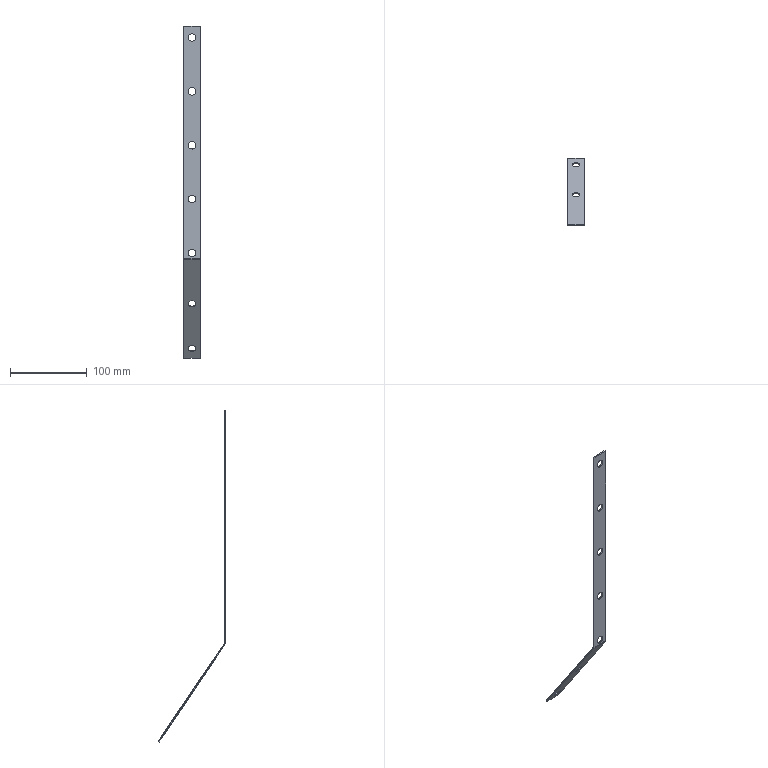Part | SolidWorks | features ICE 2, FlatPattern 1, SMBaseFlange 1, SheetMetal 1 | 1 solid | 28 faces | box 22 x 88.001 x 431.5 mm | volume 15223 mm3 | cylinder 16 | plane 12 | commonest cylinder face diameters 10 x14 3 x1 6.2 x1
STEP:
#1=CARTESIAN_POINT('',(0.,81.083,-120.21));
#2=VERTEX_POINT('',#1);
#3=CARTESIAN_POINT('',(0.,75.491,-111.92));
#4=VERTEX_POINT('',#3);
#5=CARTESIAN_POINT('',(0.,78.287,-116.065));
#6=DIRECTION('',(0.,0.829,0.5592));
#7=DIRECTION('',(0.,-0.5592,0.829));
#8=AXIS2_PLACEMENT_3D('',#5,#6,#7);
#9=CIRCLE('',#8,5.);
#10=EDGE_CURVE('',#2,#4,#9,.T.);
#11=ORIENTED_EDGE('',*,*,#10,.F.);
#12=CARTESIAN_POINT('',(0.,82.409,-119.316));
#13=VERTEX_POINT('',#12);
#14=CARTESIAN_POINT('',(0.,21.511,-160.392));
#15=DIRECTION('',(0.,0.829,0.5592));
#16=VECTOR('',#15,1000.);
#17=LINE('',#14,#16);
#18=EDGE_CURVE('',#2,#13,#17,.T.);
#19=ORIENTED_EDGE('',*,*,#18,.T.);
#20=CARTESIAN_POINT('',(0.,76.818,-111.025));
#21=VERTEX_POINT('',#20);
#22=CARTESIAN_POINT('',(0.,79.613,-115.171));
#23=DIRECTION('',(0.,0.829,0.5592));
#24=DIRECTION('',(0.,-0.5592,0.829));
#25=AXIS2_PLACEMENT_3D('',#22,#23,#24);
#26=CIRCLE('',#25,5.);
#27=EDGE_CURVE('',#13,#21,#26,.T.);
#28=ORIENTED_EDGE('',*,*,#27,.T.);
#29=CARTESIAN_POINT('',(0.,15.919,-152.102));
#30=DIRECTION('',(0.,0.829,0.5592));
#31=VECTOR('',#30,1000.);
#32=LINE('',#29,#31);
#33=EDGE_CURVE('',#4,#21,#32,.T.);
#34=ORIENTED_EDGE('',*,*,#33,.F.);
#35=EDGE_LOOP('',(#11,#19,#28,#34));
#36=FACE_OUTER_BOUND('',#35,.T.);
#37=CARTESIAN_POINT('',(0.,18.715,-156.247));
#38=DIRECTION('',(0.,0.829,0.5592));
#39=DIRECTION('',(0.,-0.5592,0.829));
#40=AXIS2_PLACEMENT_3D('',#37,#38,#39);
#41=CYLINDRICAL_SURFACE('',#40,5.);
#42=ADVANCED_FACE('',(#36),#41,.F.);
#43=CARTESIAN_POINT('',(0.,41.939,-62.178));
#44=VERTEX_POINT('',#43);
#45=CARTESIAN_POINT('',(0.,36.348,-53.887));
#46=VERTEX_POINT('',#45);
#47=CARTESIAN_POINT('',(0.,39.144,-58.033));
#48=DIRECTION('',(0.,0.829,0.5592));
#49=DIRECTION('',(0.,-0.5592,0.829));
#50=AXIS2_PLACEMENT_3D('',#47,#48,#49);
#51=CIRCLE('',#50,5.);
#52=EDGE_CURVE('',#44,#46,#51,.T.);
#53=ORIENTED_EDGE('',*,*,#52,.F.);
#54=CARTESIAN_POINT('',(0.,43.266,-61.283));
#55=VERTEX_POINT('',#54);
#56=CARTESIAN_POINT('',(0.,-17.632,-102.359));
#57=DIRECTION('',(0.,0.829,0.5592));
#58=VECTOR('',#57,1000.);
#59=LINE('',#56,#58);
#60=EDGE_CURVE('',#44,#55,#59,.T.);
#61=ORIENTED_EDGE('',*,*,#60,.T.);
#62=CARTESIAN_POINT('',(0.,37.674,-52.993));
#63=VERTEX_POINT('',#62);
#64=CARTESIAN_POINT('',(0.,40.47,-57.138));
#65=DIRECTION('',(0.,0.829,0.5592));
#66=DIRECTION('',(0.,-0.5592,0.829));
#67=AXIS2_PLACEMENT_3D('',#64,#65,#66);
#68=CIRCLE('',#67,5.);
#69=EDGE_CURVE('',#55,#63,#68,.T.);
#70=ORIENTED_EDGE('',*,*,#69,.T.);
#71=CARTESIAN_POINT('',(0.,-23.224,-94.069));
#72=DIRECTION('',(0.,0.829,0.5592));
#73=VECTOR('',#72,1000.);
#74=LINE('',#71,#73);
#75=EDGE_CURVE('',#46,#63,#74,.T.);
#76=ORIENTED_EDGE('',*,*,#75,.F.);
#77=EDGE_LOOP('',(#53,#61,#70,#76));
#78=FACE_OUTER_BOUND('',#77,.T.);
#79=CARTESIAN_POINT('',(0.,-20.428,-98.214));
#80=DIRECTION('',(0.,0.829,0.5592));
#81=DIRECTION('',(0.,-0.5592,0.829));
#82=AXIS2_PLACEMENT_3D('',#79,#80,#81);
#83=CYLINDRICAL_SURFACE('',#82,5.);
#84=ADVANCED_FACE('',(#78),#83,.F.);
#85=CARTESIAN_POINT('',(0.,0.,283.));
#86=VERTEX_POINT('',#85);
#87=CARTESIAN_POINT('',(0.,0.,293.));
#88=VERTEX_POINT('',#87);
#89=CARTESIAN_POINT('',(0.,0.,288.));
#90=DIRECTION('',(0.,1.,0.));
#91=DIRECTION('',(0.,0.,1.));
#92=AXIS2_PLACEMENT_3D('',#89,#90,#91);
#93=CIRCLE('',#92,5.);
#94=EDGE_CURVE('',#86,#88,#93,.T.);
#95=ORIENTED_EDGE('',*,*,#94,.F.);
#96=CARTESIAN_POINT('',(0.,1.6,283.));
#97=VERTEX_POINT('',#96);
#98=CARTESIAN_POINT('',(0.,0.,283.));
#99=DIRECTION('',(0.,1.,0.));
#100=VECTOR('',#99,1000.);
#101=LINE('',#98,#100);
#102=EDGE_CURVE('',#86,#97,#101,.T.);
#103=ORIENTED_EDGE('',*,*,#102,.T.);
#104=CARTESIAN_POINT('',(0.,1.6,293.));
#105=VERTEX_POINT('',#104);
#106=CARTESIAN_POINT('',(0.,1.6,288.));
#107=DIRECTION('',(0.,1.,0.));
#108=DIRECTION('',(0.,0.,1.));
#109=AXIS2_PLACEMENT_3D('',#106,#107,#108);
#110=CIRCLE('',#109,5.);
#111=EDGE_CURVE('',#97,#105,#110,.T.);
#112=ORIENTED_EDGE('',*,*,#111,.T.);
#113=CARTESIAN_POINT('',(0.,0.,293.));
#114=DIRECTION('',(0.,1.,0.));
#115=VECTOR('',#114,1000.);
#116=LINE('',#113,#115);
#117=EDGE_CURVE('',#88,#105,#116,.T.);
#118=ORIENTED_EDGE('',*,*,#117,.F.);
#119=EDGE_LOOP('',(#95,#103,#112,#118));
#120=FACE_OUTER_BOUND('',#119,.T.);
#121=CARTESIAN_POINT('',(0.,0.,288.));
#122=DIRECTION('',(0.,1.,0.));
#123=DIRECTION('',(0.,0.,1.));
#124=AXIS2_PLACEMENT_3D('',#121,#122,#123);
#125=CYLINDRICAL_SURFACE('',#124,5.);
#126=ADVANCED_FACE('',(#120),#125,.F.);
#127=CARTESIAN_POINT('',(0.,0.,213.));
#128=VERTEX_POINT('',#127);
#129=CARTESIAN_POINT('',(0.,0.,223.));
#130=VERTEX_POINT('',#129);
#131=CARTESIAN_POINT('',(0.,0.,218.));
#132=DIRECTION('',(0.,1.,0.));
#133=DIRECTION('',(0.,0.,1.));
#134=AXIS2_PLACEMENT_3D('',#131,#132,#133);
#135=CIRCLE('',#134,5.);
#136=EDGE_CURVE('',#128,#130,#135,.T.);
#137=ORIENTED_EDGE('',*,*,#136,.F.);
#138=CARTESIAN_POINT('',(0.,1.6,213.));
#139=VERTEX_POINT('',#138);
#140=CARTESIAN_POINT('',(0.,0.,213.));
#141=DIRECTION('',(0.,1.,0.));
#142=VECTOR('',#141,1000.);
#143=LINE('',#140,#142);
#144=EDGE_CURVE('',#128,#139,#143,.T.);
#145=ORIENTED_EDGE('',*,*,#144,.T.);
#146=CARTESIAN_POINT('',(0.,1.6,223.));
#147=VERTEX_POINT('',#146);
#148=CARTESIAN_POINT('',(0.,1.6,218.));
#149=DIRECTION('',(0.,1.,0.));
#150=DIRECTION('',(0.,0.,1.));
#151=AXIS2_PLACEMENT_3D('',#148,#149,#150);
#152=CIRCLE('',#151,5.);
#153=EDGE_CURVE('',#139,#147,#152,.T.);
#154=ORIENTED_EDGE('',*,*,#153,.T.);
#155=CARTESIAN_POINT('',(0.,0.,223.));
#156=DIRECTION('',(0.,1.,0.));
#157=VECTOR('',#156,1000.);
#158=LINE('',#155,#157);
#159=EDGE_CURVE('',#130,#147,#158,.T.);
#160=ORIENTED_EDGE('',*,*,#159,.F.);
#161=EDGE_LOOP('',(#137,#145,#154,#160));
#162=FACE_OUTER_BOUND('',#161,.T.);
#163=CARTESIAN_POINT('',(0.,0.,218.));
#164=DIRECTION('',(0.,1.,0.));
#165=DIRECTION('',(0.,0.,1.));
#166=AXIS2_PLACEMENT_3D('',#163,#164,#165);
#167=CYLINDRICAL_SURFACE('',#166,5.);
#168=ADVANCED_FACE('',(#162),#167,.F.);
#169=CARTESIAN_POINT('',(0.,0.,143.));
#170=VERTEX_POINT('',#169);
#171=CARTESIAN_POINT('',(0.,0.,153.));
#172=VERTEX_POINT('',#171);
#173=CARTESIAN_POINT('',(0.,0.,148.));
#174=DIRECTION('',(0.,1.,0.));
#175=DIRECTION('',(0.,0.,1.));
#176=AXIS2_PLACEMENT_3D('',#173,#174,#175);
#177=CIRCLE('',#176,5.);
#178=EDGE_CURVE('',#170,#172,#177,.T.);
#179=ORIENTED_EDGE('',*,*,#178,.F.);
#180=CARTESIAN_POINT('',(0.,1.6,143.));
#181=VERTEX_POINT('',#180);
#182=CARTESIAN_POINT('',(0.,0.,143.));
#183=DIRECTION('',(0.,1.,0.));
#184=VECTOR('',#183,1000.);
#185=LINE('',#182,#184);
#186=EDGE_CURVE('',#170,#181,#185,.T.);
#187=ORIENTED_EDGE('',*,*,#186,.T.);
#188=CARTESIAN_POINT('',(0.,1.6,153.));
#189=VERTEX_POINT('',#188);
#190=CARTESIAN_POINT('',(0.,1.6,148.));
#191=DIRECTION('',(0.,1.,0.));
#192=DIRECTION('',(0.,0.,1.));
#193=AXIS2_PLACEMENT_3D('',#190,#191,#192);
#194=CIRCLE('',#193,5.);
#195=EDGE_CURVE('',#181,#189,#194,.T.);
#196=ORIENTED_EDGE('',*,*,#195,.T.);
#197=CARTESIAN_POINT('',(0.,0.,153.));
#198=DIRECTION('',(0.,1.,0.));
#199=VECTOR('',#198,1000.);
#200=LINE('',#197,#199);
#201=EDGE_CURVE('',#172,#189,#200,.T.);
#202=ORIENTED_EDGE('',*,*,#201,.F.);
#203=EDGE_LOOP('',(#179,#187,#196,#202));
#204=FACE_OUTER_BOUND('',#203,.T.);
#205=CARTESIAN_POINT('',(0.,0.,148.));
#206=DIRECTION('',(0.,1.,0.));
#207=DIRECTION('',(0.,0.,1.));
#208=AXIS2_PLACEMENT_3D('',#205,#206,#207);
#209=CYLINDRICAL_SURFACE('',#208,5.);
#210=ADVANCED_FACE('',(#204),#209,.F.);
#211=CARTESIAN_POINT('',(0.,0.,73.));
#212=VERTEX_POINT('',#211);
#213=CARTESIAN_POINT('',(0.,0.,83.));
#214=VERTEX_POINT('',#213);
#215=CARTESIAN_POINT('',(0.,0.,78.));
#216=DIRECTION('',(0.,1.,0.));
#217=DIRECTION('',(0.,0.,1.));
#218=AXIS2_PLACEMENT_3D('',#215,#216,#217);
#219=CIRCLE('',#218,5.);
#220=EDGE_CURVE('',#212,#214,#219,.T.);
#221=ORIENTED_EDGE('',*,*,#220,.F.);
#222=CARTESIAN_POINT('',(0.,1.6,73.));
#223=VERTEX_POINT('',#222);
#224=CARTESIAN_POINT('',(0.,0.,73.));
#225=DIRECTION('',(0.,1.,0.));
#226=VECTOR('',#225,1000.);
#227=LINE('',#224,#226);
#228=EDGE_CURVE('',#212,#223,#227,.T.);
#229=ORIENTED_EDGE('',*,*,#228,.T.);
#230=CARTESIAN_POINT('',(0.,1.6,83.));
#231=VERTEX_POINT('',#230);
#232=CARTESIAN_POINT('',(0.,1.6,78.));
#233=DIRECTION('',(0.,1.,0.));
#234=DIRECTION('',(0.,0.,1.));
#235=AXIS2_PLACEMENT_3D('',#232,#233,#234);
#236=CIRCLE('',#235,5.);
#237=EDGE_CURVE('',#223,#231,#236,.T.);
#238=ORIENTED_EDGE('',*,*,#237,.T.);
#239=CARTESIAN_POINT('',(0.,0.,83.));
#240=DIRECTION('',(0.,1.,0.));
#241=VECTOR('',#240,1000.);
#242=LINE('',#239,#241);
#243=EDGE_CURVE('',#214,#231,#242,.T.);
#244=ORIENTED_EDGE('',*,*,#243,.F.);
#245=EDGE_LOOP('',(#221,#229,#238,#244));
#246=FACE_OUTER_BOUND('',#245,.T.);
#247=CARTESIAN_POINT('',(0.,0.,78.));
#248=DIRECTION('',(0.,1.,0.));
#249=DIRECTION('',(0.,0.,1.));
#250=AXIS2_PLACEMENT_3D('',#247,#248,#249);
#251=CYLINDRICAL_SURFACE('',#250,5.);
#252=ADVANCED_FACE('',(#246),#251,.F.);
#253=CARTESIAN_POINT('',(0.,0.,3.));
#254=VERTEX_POINT('',#253);
#255=CARTESIAN_POINT('',(0.,0.,13.));
#256=VERTEX_POINT('',#255);
#257=CARTESIAN_POINT('',(0.,0.,8.));
#258=DIRECTION('',(0.,1.,0.));
#259=DIRECTION('',(0.,0.,1.));
#260=AXIS2_PLACEMENT_3D('',#257,#258,#259);
#261=CIRCLE('',#260,5.);
#262=EDGE_CURVE('',#254,#256,#261,.T.);
#263=ORIENTED_EDGE('',*,*,#262,.F.);
#264=CARTESIAN_POINT('',(0.,1.6,3.));
#265=VERTEX_POINT('',#264);
#266=CARTESIAN_POINT('',(0.,0.,3.));
#267=DIRECTION('',(0.,1.,0.));
#268=VECTOR('',#267,1000.);
#269=LINE('',#266,#268);
#270=EDGE_CURVE('',#254,#265,#269,.T.);
#271=ORIENTED_EDGE('',*,*,#270,.T.);
#272=CARTESIAN_POINT('',(0.,1.6,13.));
#273=VERTEX_POINT('',#272);
#274=CARTESIAN_POINT('',(0.,1.6,8.));
#275=DIRECTION('',(0.,1.,0.));
#276=DIRECTION('',(0.,0.,1.));
#277=AXIS2_PLACEMENT_3D('',#274,#275,#276);
#278=CIRCLE('',#277,5.);
#279=EDGE_CURVE('',#265,#273,#278,.T.);
#280=ORIENTED_EDGE('',*,*,#279,.T.);
#281=CARTESIAN_POINT('',(0.,0.,13.));
#282=DIRECTION('',(0.,1.,0.));
#283=VECTOR('',#282,1000.);
#284=LINE('',#281,#283);
#285=EDGE_CURVE('',#256,#273,#284,.T.);
#286=ORIENTED_EDGE('',*,*,#285,.F.);
#287=EDGE_LOOP('',(#263,#271,#280,#286));
#288=FACE_OUTER_BOUND('',#287,.T.);
#289=CARTESIAN_POINT('',(0.,0.,8.));
#290=DIRECTION('',(0.,1.,0.));
#291=DIRECTION('',(0.,0.,1.));
#292=AXIS2_PLACEMENT_3D('',#289,#290,#291);
#293=CYLINDRICAL_SURFACE('',#292,5.);
#294=ADVANCED_FACE('',(#288),#293,.F.);
#295=CARTESIAN_POINT('',(11.,0.,0.9478));
#296=VERTEX_POINT('',#295);
#297=CARTESIAN_POINT('',(11.,1.6,0.9478));
#298=VERTEX_POINT('',#297);
#299=CARTESIAN_POINT('',(11.,0.,0.9478));
#300=DIRECTION('',(0.,1.,0.));
#301=VECTOR('',#300,1000.);
#302=LINE('',#299,#301);
#303=EDGE_CURVE('',#296,#298,#302,.T.);
#304=ORIENTED_EDGE('',*,*,#303,.F.);
#305=CARTESIAN_POINT('',(11.,0.53,-0.7857));
#306=VERTEX_POINT('',#305);
#307=CARTESIAN_POINT('',(11.,3.1,0.9478));
#308=DIRECTION('',(1.,0.,0.));
#309=DIRECTION('',(0.,0.,1.));
#310=AXIS2_PLACEMENT_3D('',#307,#308,#309);
#311=CIRCLE('',#310,3.1);
#312=EDGE_CURVE('',#296,#306,#311,.T.);
#313=ORIENTED_EDGE('',*,*,#312,.T.);
#314=CARTESIAN_POINT('',(11.,1.856,0.109));
#315=VERTEX_POINT('',#314);
#316=CARTESIAN_POINT('',(11.,1.856,0.109));
#317=DIRECTION('',(0.,-0.829,-0.5592));
#318=VECTOR('',#317,1000.);
#319=LINE('',#316,#318);
#320=EDGE_CURVE('',#315,#306,#319,.T.);
#321=ORIENTED_EDGE('',*,*,#320,.F.);
#322=CARTESIAN_POINT('',(11.,3.1,0.9478));
#323=DIRECTION('',(1.,0.,0.));
#324=DIRECTION('',(0.,0.,-1.));
#325=AXIS2_PLACEMENT_3D('',#322,#323,#324);
#326=CIRCLE('',#325,1.5);
#327=EDGE_CURVE('',#298,#315,#326,.T.);
#328=ORIENTED_EDGE('',*,*,#327,.F.);
#329=EDGE_LOOP('',(#304,#313,#321,#328));
#330=FACE_OUTER_BOUND('',#329,.T.);
#331=CARTESIAN_POINT('',(11.,0.,0.9478));
#332=DIRECTION('',(1.,0.,0.));
#333=DIRECTION('',(0.,0.,-1.));
#334=AXIS2_PLACEMENT_3D('',#331,#332,#333);
#335=PLANE('',#334);
#336=ADVANCED_FACE('',(#330),#335,.T.);
#337=CARTESIAN_POINT('',(11.,0.,303.));
#338=VERTEX_POINT('',#337);
#339=CARTESIAN_POINT('',(11.,0.,0.));
#340=DIRECTION('',(0.,0.,-1.));
#341=VECTOR('',#340,1000.);
#342=LINE('',#339,#341);
#343=EDGE_CURVE('',#338,#296,#342,.T.);
#344=ORIENTED_EDGE('',*,*,#343,.T.);
#345=ORIENTED_EDGE('',*,*,#303,.T.);
#346=CARTESIAN_POINT('',(11.,1.6,303.));
#347=VERTEX_POINT('',#346);
#348=CARTESIAN_POINT('',(11.,1.6,0.));
#349=DIRECTION('',(0.,0.,-1.));
#350=VECTOR('',#349,1000.);
#351=LINE('',#348,#350);
#352=EDGE_CURVE('',#347,#298,#351,.T.);
#353=ORIENTED_EDGE('',*,*,#352,.F.);
#354=CARTESIAN_POINT('',(11.,0.,303.));
#355=DIRECTION('',(0.,1.,0.));
#356=VECTOR('',#355,1000.);
#357=LINE('',#354,#356);
#358=EDGE_CURVE('',#338,#347,#357,.T.);
#359=ORIENTED_EDGE('',*,*,#358,.F.);
#360=EDGE_LOOP('',(#344,#345,#353,#359));
#361=FACE_OUTER_BOUND('',#360,.T.);
#362=CARTESIAN_POINT('',(11.,1.856,0.109));
#363=DIRECTION('',(1.,0.,0.));
#364=DIRECTION('',(0.,0.,-1.));
#365=AXIS2_PLACEMENT_3D('',#362,#363,#364);
#366=PLANE('',#365);
#367=ADVANCED_FACE('',(#361),#366,.T.);
#368=CARTESIAN_POINT('',(-11.,0.53,-0.7857));
#369=VERTEX_POINT('',#368);
#370=CARTESIAN_POINT('',(-11.,1.856,0.109));
#371=VERTEX_POINT('',#370);
#372=CARTESIAN_POINT('',(-11.,0.53,-0.7857));
#373=DIRECTION('',(0.,0.829,0.5592));
#374=VECTOR('',#373,1000.);
#375=LINE('',#372,#374);
#376=EDGE_CURVE('',#369,#371,#375,.T.);
#377=ORIENTED_EDGE('',*,*,#376,.F.);
#378=CARTESIAN_POINT('',(-11.,0.,0.9478));
#379=VERTEX_POINT('',#378);
#380=CARTESIAN_POINT('',(-11.,3.1,0.9478));
#381=DIRECTION('',(1.,0.,0.));
#382=DIRECTION('',(0.,0.,1.));
#383=AXIS2_PLACEMENT_3D('',#380,#381,#382);
#384=CIRCLE('',#383,3.1);
#385=EDGE_CURVE('',#379,#369,#384,.T.);
#386=ORIENTED_EDGE('',*,*,#385,.F.);
#387=CARTESIAN_POINT('',(-11.,1.6,0.9478));
#388=VERTEX_POINT('',#387);
#389=CARTESIAN_POINT('',(-11.,1.6,0.9478));
#390=DIRECTION('',(0.,-1.,0.));
#391=VECTOR('',#390,1000.);
#392=LINE('',#389,#391);
#393=EDGE_CURVE('',#388,#379,#392,.T.);
#394=ORIENTED_EDGE('',*,*,#393,.F.);
#395=CARTESIAN_POINT('',(-11.,3.1,0.9478));
#396=DIRECTION('',(1.,0.,0.));
#397=DIRECTION('',(0.,0.,-1.));
#398=AXIS2_PLACEMENT_3D('',#395,#396,#397);
#399=CIRCLE('',#398,1.5);
#400=EDGE_CURVE('',#388,#371,#399,.T.);
#401=ORIENTED_EDGE('',*,*,#400,.T.);
#402=EDGE_LOOP('',(#377,#386,#394,#401));
#403=FACE_OUTER_BOUND('',#402,.T.);
#404=CARTESIAN_POINT('',(-11.,0.53,-0.7857));
#405=DIRECTION('',(-1.,0.,0.));
#406=DIRECTION('',(0.,0.,1.));
#407=AXIS2_PLACEMENT_3D('',#404,#405,#406);
#408=PLANE('',#407);
#409=ADVANCED_FACE('',(#403),#408,.T.);
#410=CARTESIAN_POINT('',(-11.,86.674,-128.5));
#411=VERTEX_POINT('',#410);
#412=CARTESIAN_POINT('',(-11.,0.,0.));
#413=DIRECTION('',(0.,0.5592,-0.829));
#414=VECTOR('',#413,1000.);
#415=LINE('',#412,#414);
#416=EDGE_CURVE('',#369,#411,#415,.T.);
#417=ORIENTED_EDGE('',*,*,#416,.F.);
#418=ORIENTED_EDGE('',*,*,#376,.T.);
#419=CARTESIAN_POINT('',(-11.,88.001,-127.605));
#420=VERTEX_POINT('',#419);
#421=CARTESIAN_POINT('',(-11.,1.326,0.8947));
#422=DIRECTION('',(0.,0.5592,-0.829));
#423=VECTOR('',#422,1000.);
#424=LINE('',#421,#423);
#425=EDGE_CURVE('',#371,#420,#424,.T.);
#426=ORIENTED_EDGE('',*,*,#425,.T.);
#427=CARTESIAN_POINT('',(-11.,88.001,-127.605));
#428=DIRECTION('',(0.,-0.829,-0.5592));
#429=VECTOR('',#428,1000.);
#430=LINE('',#427,#429);
#431=EDGE_CURVE('',#420,#411,#430,.T.);
#432=ORIENTED_EDGE('',*,*,#431,.T.);
#433=EDGE_LOOP('',(#417,#418,#426,#432));
#434=FACE_OUTER_BOUND('',#433,.T.);
#435=CARTESIAN_POINT('',(-11.,1.6,0.9478));
#436=DIRECTION('',(-1.,0.,0.));
#437=DIRECTION('',(0.,0.,1.));
#438=AXIS2_PLACEMENT_3D('',#435,#436,#437);
#439=PLANE('',#438);
#440=ADVANCED_FACE('',(#434),#439,.T.);
#441=CARTESIAN_POINT('',(0.,78.287,-116.065));
#442=DIRECTION('',(0.,0.829,0.5592));
#443=DIRECTION('',(0.,-0.5592,0.829));
#444=AXIS2_PLACEMENT_3D('',#441,#442,#443);
#445=CIRCLE('',#444,5.);
#446=EDGE_CURVE('',#4,#2,#445,.T.);
#447=ORIENTED_EDGE('',*,*,#446,.T.);
#448=ORIENTED_EDGE('',*,*,#10,.T.);
#449=EDGE_LOOP('',(#447,#448));
#450=FACE_BOUND('',#449,.T.);
#451=CARTESIAN_POINT('',(0.,39.144,-58.033));
#452=DIRECTION('',(0.,0.829,0.5592));
#453=DIRECTION('',(0.,-0.5592,0.829));
#454=AXIS2_PLACEMENT_3D('',#451,#452,#453);
#455=CIRCLE('',#454,5.);
#456=EDGE_CURVE('',#46,#44,#455,.T.);
#457=ORIENTED_EDGE('',*,*,#456,.T.);
#458=ORIENTED_EDGE('',*,*,#52,.T.);
#459=EDGE_LOOP('',(#457,#458));
#460=FACE_BOUND('',#459,.T.);
#461=ORIENTED_EDGE('',*,*,#416,.T.);
#462=CARTESIAN_POINT('',(11.,86.674,-128.5));
#463=VERTEX_POINT('',#462);
#464=CARTESIAN_POINT('',(11.,86.674,-128.5));
#465=DIRECTION('',(-1.,0.,0.));
#466=VECTOR('',#465,1000.);
#467=LINE('',#464,#466);
#468=EDGE_CURVE('',#463,#411,#467,.T.);
#469=ORIENTED_EDGE('',*,*,#468,.F.);
#470=CARTESIAN_POINT('',(11.,0.,0.));
#471=DIRECTION('',(0.,0.5592,-0.829));
#472=VECTOR('',#471,1000.);
#473=LINE('',#470,#472);
#474=EDGE_CURVE('',#306,#463,#473,.T.);
#475=ORIENTED_EDGE('',*,*,#474,.F.);
#476=CARTESIAN_POINT('',(11.,0.53,-0.7857));
#477=DIRECTION('',(-1.,0.,0.));
#478=VECTOR('',#477,1000.);
#479=LINE('',#476,#478);
#480=EDGE_CURVE('',#306,#369,#479,.T.);
#481=ORIENTED_EDGE('',*,*,#480,.T.);
#482=EDGE_LOOP('',(#461,#469,#475,#481));
#483=FACE_OUTER_BOUND('',#482,.T.);
#484=CARTESIAN_POINT('',(11.,0.,0.));
#485=DIRECTION('',(0.,0.829,0.5592));
#486=DIRECTION('',(0.,-0.5592,0.829));
#487=AXIS2_PLACEMENT_3D('',#484,#485,#486);
#488=PLANE('',#487);
#489=ADVANCED_FACE('',(#450,#460,#483),#488,.F.);
#490=ORIENTED_EDGE('',*,*,#431,.F.);
#491=CARTESIAN_POINT('',(11.,88.001,-127.605));
#492=VERTEX_POINT('',#491);
#493=CARTESIAN_POINT('',(11.,88.001,-127.605));
#494=DIRECTION('',(-1.,0.,0.));
#495=VECTOR('',#494,1000.);
#496=LINE('',#493,#495);
#497=EDGE_CURVE('',#492,#420,#496,.T.);
#498=ORIENTED_EDGE('',*,*,#497,.F.);
#499=CARTESIAN_POINT('',(11.,88.001,-127.605));
#500=DIRECTION('',(0.,-0.829,-0.5592));
#501=VECTOR('',#500,1000.);
#502=LINE('',#499,#501);
#503=EDGE_CURVE('',#492,#463,#502,.T.);
#504=ORIENTED_EDGE('',*,*,#503,.T.);
#505=ORIENTED_EDGE('',*,*,#468,.T.);
#506=EDGE_LOOP('',(#490,#498,#504,#505));
#507=FACE_OUTER_BOUND('',#506,.T.);
#508=CARTESIAN_POINT('',(11.,88.001,-127.605));
#509=DIRECTION('',(0.,0.5592,-0.829));
#510=DIRECTION('',(0.,0.829,0.5592));
#511=AXIS2_PLACEMENT_3D('',#508,#509,#510);
#512=PLANE('',#511);
#513=ADVANCED_FACE('',(#507),#512,.T.);
#514=CARTESIAN_POINT('',(0.,79.613,-115.171));
#515=DIRECTION('',(0.,0.829,0.5592));
#516=DIRECTION('',(0.,-0.5592,0.829));
#517=AXIS2_PLACEMENT_3D('',#514,#515,#516);
#518=CIRCLE('',#517,5.);
#519=EDGE_CURVE('',#21,#13,#518,.T.);
#520=ORIENTED_EDGE('',*,*,#519,.F.);
#521=ORIENTED_EDGE('',*,*,#27,.F.);
#522=EDGE_LOOP('',(#520,#521));
#523=FACE_BOUND('',#522,.T.);
#524=CARTESIAN_POINT('',(0.,40.47,-57.138));
#525=DIRECTION('',(0.,0.829,0.5592));
#526=DIRECTION('',(0.,-0.5592,0.829));
#527=AXIS2_PLACEMENT_3D('',#524,#525,#526);
#528=CIRCLE('',#527,5.);
#529=EDGE_CURVE('',#63,#55,#528,.T.);
#530=ORIENTED_EDGE('',*,*,#529,.F.);
#531=ORIENTED_EDGE('',*,*,#69,.F.);
#532=EDGE_LOOP('',(#530,#531));
#533=FACE_BOUND('',#532,.T.);
#534=ORIENTED_EDGE('',*,*,#425,.F.);
#535=CARTESIAN_POINT('',(11.,1.856,0.109));
#536=DIRECTION('',(-1.,0.,0.));
#537=VECTOR('',#536,1000.);
#538=LINE('',#535,#537);
#539=EDGE_CURVE('',#315,#371,#538,.T.);
#540=ORIENTED_EDGE('',*,*,#539,.F.);
#541=CARTESIAN_POINT('',(11.,1.326,0.8947));
#542=DIRECTION('',(0.,0.5592,-0.829));
#543=VECTOR('',#542,1000.);
#544=LINE('',#541,#543);
#545=EDGE_CURVE('',#315,#492,#544,.T.);
#546=ORIENTED_EDGE('',*,*,#545,.T.);
#547=ORIENTED_EDGE('',*,*,#497,.T.);
#548=EDGE_LOOP('',(#534,#540,#546,#547));
#549=FACE_OUTER_BOUND('',#548,.T.);
#550=CARTESIAN_POINT('',(11.,1.326,0.8947));
#551=DIRECTION('',(0.,0.829,0.5592));
#552=DIRECTION('',(0.,-0.5592,0.829));
#553=AXIS2_PLACEMENT_3D('',#550,#551,#552);
#554=PLANE('',#553);
#555=ADVANCED_FACE('',(#523,#533,#549),#554,.T.);
#556=ORIENTED_EDGE('',*,*,#400,.F.);
#557=CARTESIAN_POINT('',(11.,1.6,0.9478));
#558=DIRECTION('',(-1.,0.,0.));
#559=VECTOR('',#558,1000.);
#560=LINE('',#557,#559);
#561=EDGE_CURVE('',#298,#388,#560,.T.);
#562=ORIENTED_EDGE('',*,*,#561,.F.);
#563=ORIENTED_EDGE('',*,*,#327,.T.);
#564=ORIENTED_EDGE('',*,*,#539,.T.);
#565=EDGE_LOOP('',(#556,#562,#563,#564));
#566=FACE_OUTER_BOUND('',#565,.T.);
#567=CARTESIAN_POINT('',(11.,3.1,0.9478));
#568=DIRECTION('',(-1.,0.,0.));
#569=DIRECTION('',(0.,0.,1.));
#570=AXIS2_PLACEMENT_3D('',#567,#568,#569);
#571=CYLINDRICAL_SURFACE('',#570,1.5);
#572=ADVANCED_FACE('',(#566),#571,.F.);
#573=CARTESIAN_POINT('',(0.,1.6,288.));
#574=DIRECTION('',(0.,1.,0.));
#575=DIRECTION('',(0.,0.,1.));
#576=AXIS2_PLACEMENT_3D('',#573,#574,#575);
#577=CIRCLE('',#576,5.);
#578=EDGE_CURVE('',#105,#97,#577,.T.);
#579=ORIENTED_EDGE('',*,*,#578,.F.);
#580=ORIENTED_EDGE('',*,*,#111,.F.);
#581=EDGE_LOOP('',(#579,#580));
#582=FACE_BOUND('',#581,.T.);
#583=CARTESIAN_POINT('',(0.,1.6,218.));
#584=DIRECTION('',(0.,1.,0.));
#585=DIRECTION('',(0.,0.,1.));
#586=AXIS2_PLACEMENT_3D('',#583,#584,#585);
#587=CIRCLE('',#586,5.);
#588=EDGE_CURVE('',#147,#139,#587,.T.);
#589=ORIENTED_EDGE('',*,*,#588,.F.);
#590=ORIENTED_EDGE('',*,*,#153,.F.);
#591=EDGE_LOOP('',(#589,#590));
#592=FACE_BOUND('',#591,.T.);
#593=CARTESIAN_POINT('',(0.,1.6,148.));
#594=DIRECTION('',(0.,1.,0.));
#595=DIRECTION('',(0.,0.,1.));
#596=AXIS2_PLACEMENT_3D('',#593,#594,#595);
#597=CIRCLE('',#596,5.);
#598=EDGE_CURVE('',#189,#181,#597,.T.);
#599=ORIENTED_EDGE('',*,*,#598,.F.);
#600=ORIENTED_EDGE('',*,*,#195,.F.);
#601=EDGE_LOOP('',(#599,#600));
#602=FACE_BOUND('',#601,.T.);
#603=CARTESIAN_POINT('',(0.,1.6,78.));
#604=DIRECTION('',(0.,1.,0.));
#605=DIRECTION('',(0.,0.,1.));
#606=AXIS2_PLACEMENT_3D('',#603,#604,#605);
#607=CIRCLE('',#606,5.);
#608=EDGE_CURVE('',#231,#223,#607,.T.);
#609=ORIENTED_EDGE('',*,*,#608,.F.);
#610=ORIENTED_EDGE('',*,*,#237,.F.);
#611=EDGE_LOOP('',(#609,#610));
#612=FACE_BOUND('',#611,.T.);
#613=CARTESIAN_POINT('',(0.,1.6,8.));
#614=DIRECTION('',(0.,1.,0.));
#615=DIRECTION('',(0.,0.,1.));
#616=AXIS2_PLACEMENT_3D('',#613,#614,#615);
#617=CIRCLE('',#616,5.);
#618=EDGE_CURVE('',#273,#265,#617,.T.);
#619=ORIENTED_EDGE('',*,*,#618,.F.);
#620=ORIENTED_EDGE('',*,*,#279,.F.);
#621=EDGE_LOOP('',(#619,#620));
#622=FACE_BOUND('',#621,.T.);
#623=CARTESIAN_POINT('',(-11.,1.6,303.));
#624=VERTEX_POINT('',#623);
#625=CARTESIAN_POINT('',(-11.,1.6,0.));
#626=DIRECTION('',(0.,0.,-1.));
#627=VECTOR('',#626,1000.);
#628=LINE('',#625,#627);
#629=EDGE_CURVE('',#624,#388,#628,.T.);
#630=ORIENTED_EDGE('',*,*,#629,.F.);
#631=CARTESIAN_POINT('',(11.,1.6,303.));
#632=DIRECTION('',(-1.,0.,0.));
#633=VECTOR('',#632,1000.);
#634=LINE('',#631,#633);
#635=EDGE_CURVE('',#347,#624,#634,.T.);
#636=ORIENTED_EDGE('',*,*,#635,.F.);
#637=ORIENTED_EDGE('',*,*,#352,.T.);
#638=ORIENTED_EDGE('',*,*,#561,.T.);
#639=EDGE_LOOP('',(#630,#636,#637,#638));
#640=FACE_OUTER_BOUND('',#639,.T.);
#641=CARTESIAN_POINT('',(11.,1.6,0.));
#642=DIRECTION('',(0.,1.,0.));
#643=DIRECTION('',(0.,0.,1.));
#644=AXIS2_PLACEMENT_3D('',#641,#642,#643);
#645=PLANE('',#644);
#646=ADVANCED_FACE('',(#582,#592,#602,#612,#622,#640),#645,.T.);
#647=CARTESIAN_POINT('',(-11.,0.,303.));
#648=VERTEX_POINT('',#647);
#649=CARTESIAN_POINT('',(-11.,0.,303.));
#650=DIRECTION('',(0.,1.,0.));
#651=VECTOR('',#650,1000.);
#652=LINE('',#649,#651);
#653=EDGE_CURVE('',#648,#624,#652,.T.);
#654=ORIENTED_EDGE('',*,*,#653,.F.);
#655=CARTESIAN_POINT('',(11.,0.,303.));
#656=DIRECTION('',(-1.,0.,0.));
#657=VECTOR('',#656,1000.);
#658=LINE('',#655,#657);
#659=EDGE_CURVE('',#338,#648,#658,.T.);
#660=ORIENTED_EDGE('',*,*,#659,.F.);
#661=ORIENTED_EDGE('',*,*,#358,.T.);
#662=ORIENTED_EDGE('',*,*,#635,.T.);
#663=EDGE_LOOP('',(#654,#660,#661,#662));
#664=FACE_OUTER_BOUND('',#663,.T.);
#665=CARTESIAN_POINT('',(11.,0.,303.));
#666=DIRECTION('',(0.,0.,1.));
#667=DIRECTION('',(1.,0.,0.));
#668=AXIS2_PLACEMENT_3D('',#665,#666,#667);
#669=PLANE('',#668);
#670=ADVANCED_FACE('',(#664),#669,.T.);
#671=CARTESIAN_POINT('',(0.,0.,288.));
#672=DIRECTION('',(0.,1.,0.));
#673=DIRECTION('',(0.,0.,1.));
#674=AXIS2_PLACEMENT_3D('',#671,#672,#673);
#675=CIRCLE('',#674,5.);
#676=EDGE_CURVE('',#88,#86,#675,.T.);
#677=ORIENTED_EDGE('',*,*,#676,.T.);
#678=ORIENTED_EDGE('',*,*,#94,.T.);
#679=EDGE_LOOP('',(#677,#678));
#680=FACE_BOUND('',#679,.T.);
#681=CARTESIAN_POINT('',(0.,0.,218.));
#682=DIRECTION('',(0.,1.,0.));
#683=DIRECTION('',(0.,0.,1.));
#684=AXIS2_PLACEMENT_3D('',#681,#682,#683);
#685=CIRCLE('',#684,5.);
#686=EDGE_CURVE('',#130,#128,#685,.T.);
#687=ORIENTED_EDGE('',*,*,#686,.T.);
#688=ORIENTED_EDGE('',*,*,#136,.T.);
#689=EDGE_LOOP('',(#687,#688));
#690=FACE_BOUND('',#689,.T.);
#691=CARTESIAN_POINT('',(0.,0.,148.));
#692=DIRECTION('',(0.,1.,0.));
#693=DIRECTION('',(0.,0.,1.));
#694=AXIS2_PLACEMENT_3D('',#691,#692,#693);
#695=CIRCLE('',#694,5.);
#696=EDGE_CURVE('',#172,#170,#695,.T.);
#697=ORIENTED_EDGE('',*,*,#696,.T.);
#698=ORIENTED_EDGE('',*,*,#178,.T.);
#699=EDGE_LOOP('',(#697,#698));
#700=FACE_BOUND('',#699,.T.);
#701=CARTESIAN_POINT('',(0.,0.,78.));
#702=DIRECTION('',(0.,1.,0.));
#703=DIRECTION('',(0.,0.,1.));
#704=AXIS2_PLACEMENT_3D('',#701,#702,#703);
#705=CIRCLE('',#704,5.);
#706=EDGE_CURVE('',#214,#212,#705,.T.);
#707=ORIENTED_EDGE('',*,*,#706,.T.);
#708=ORIENTED_EDGE('',*,*,#220,.T.);
#709=EDGE_LOOP('',(#707,#708));
#710=FACE_BOUND('',#709,.T.);
#711=CARTESIAN_POINT('',(0.,0.,8.));
#712=DIRECTION('',(0.,1.,0.));
#713=DIRECTION('',(0.,0.,1.));
#714=AXIS2_PLACEMENT_3D('',#711,#712,#713);
#715=CIRCLE('',#714,5.);
#716=EDGE_CURVE('',#256,#254,#715,.T.);
#717=ORIENTED_EDGE('',*,*,#716,.T.);
#718=ORIENTED_EDGE('',*,*,#262,.T.);
#719=EDGE_LOOP('',(#717,#718));
#720=FACE_BOUND('',#719,.T.);
#721=CARTESIAN_POINT('',(-11.,0.,0.));
#722=DIRECTION('',(0.,0.,-1.));
#723=VECTOR('',#722,1000.);
#724=LINE('',#721,#723);
#725=EDGE_CURVE('',#648,#379,#724,.T.);
#726=ORIENTED_EDGE('',*,*,#725,.T.);
#727=CARTESIAN_POINT('',(11.,0.,0.9478));
#728=DIRECTION('',(-1.,0.,0.));
#729=VECTOR('',#728,1000.);
#730=LINE('',#727,#729);
#731=EDGE_CURVE('',#296,#379,#730,.T.);
#732=ORIENTED_EDGE('',*,*,#731,.F.);
#733=ORIENTED_EDGE('',*,*,#343,.F.);
#734=ORIENTED_EDGE('',*,*,#659,.T.);
#735=EDGE_LOOP('',(#726,#732,#733,#734));
#736=FACE_OUTER_BOUND('',#735,.T.);
#737=CARTESIAN_POINT('',(11.,0.,0.));
#738=DIRECTION('',(0.,1.,0.));
#739=DIRECTION('',(0.,0.,1.));
#740=AXIS2_PLACEMENT_3D('',#737,#738,#739);
#741=PLANE('',#740);
#742=ADVANCED_FACE('',(#680,#690,#700,#710,#720,#736),#741,.F.);
#743=ORIENTED_EDGE('',*,*,#385,.T.);
#744=ORIENTED_EDGE('',*,*,#480,.F.);
#745=ORIENTED_EDGE('',*,*,#312,.F.);
#746=ORIENTED_EDGE('',*,*,#731,.T.);
#747=EDGE_LOOP('',(#743,#744,#745,#746));
#748=FACE_OUTER_BOUND('',#747,.T.);
#749=CARTESIAN_POINT('',(11.,3.1,0.9478));
#750=DIRECTION('',(-1.,0.,0.));
#751=DIRECTION('',(0.,0.,1.));
#752=AXIS2_PLACEMENT_3D('',#749,#750,#751);
#753=CYLINDRICAL_SURFACE('',#752,3.1);
#754=ADVANCED_FACE('',(#748),#753,.T.);
#755=ORIENTED_EDGE('',*,*,#474,.T.);
#756=ORIENTED_EDGE('',*,*,#503,.F.);
#757=ORIENTED_EDGE('',*,*,#545,.F.);
#758=ORIENTED_EDGE('',*,*,#320,.T.);
#759=EDGE_LOOP('',(#755,#756,#757,#758));
#760=FACE_OUTER_BOUND('',#759,.T.);
#761=CARTESIAN_POINT('',(11.,3.1,0.9478));
#762=DIRECTION('',(1.,0.,0.));
#763=DIRECTION('',(0.,0.,-1.));
#764=AXIS2_PLACEMENT_3D('',#761,#762,#763);
#765=PLANE('',#764);
#766=ADVANCED_FACE('',(#760),#765,.T.);
#767=ORIENTED_EDGE('',*,*,#629,.T.);
#768=ORIENTED_EDGE('',*,*,#393,.T.);
#769=ORIENTED_EDGE('',*,*,#725,.F.);
#770=ORIENTED_EDGE('',*,*,#653,.T.);
#771=EDGE_LOOP('',(#767,#768,#769,#770));
#772=FACE_OUTER_BOUND('',#771,.T.);
#773=CARTESIAN_POINT('',(-11.,3.1,0.9478));
#774=DIRECTION('',(1.,0.,0.));
#775=DIRECTION('',(0.,0.,-1.));
#776=AXIS2_PLACEMENT_3D('',#773,#774,#775);
#777=PLANE('',#776);
#778=ADVANCED_FACE('',(#772),#777,.F.);
#779=ORIENTED_EDGE('',*,*,#270,.F.);
#780=ORIENTED_EDGE('',*,*,#716,.F.);
#781=ORIENTED_EDGE('',*,*,#285,.T.);
#782=ORIENTED_EDGE('',*,*,#618,.T.);
#783=EDGE_LOOP('',(#779,#780,#781,#782));
#784=FACE_OUTER_BOUND('',#783,.T.);
#785=CARTESIAN_POINT('',(0.,0.,8.));
#786=DIRECTION('',(0.,1.,0.));
#787=DIRECTION('',(0.,0.,1.));
#788=AXIS2_PLACEMENT_3D('',#785,#786,#787);
#789=CYLINDRICAL_SURFACE('',#788,5.);
#790=ADVANCED_FACE('',(#784),#789,.F.);
#791=ORIENTED_EDGE('',*,*,#228,.F.);
#792=ORIENTED_EDGE('',*,*,#706,.F.);
#793=ORIENTED_EDGE('',*,*,#243,.T.);
#794=ORIENTED_EDGE('',*,*,#608,.T.);
#795=EDGE_LOOP('',(#791,#792,#793,#794));
#796=FACE_OUTER_BOUND('',#795,.T.);
#797=CARTESIAN_POINT('',(0.,0.,78.));
#798=DIRECTION('',(0.,1.,0.));
#799=DIRECTION('',(0.,0.,1.));
#800=AXIS2_PLACEMENT_3D('',#797,#798,#799);
#801=CYLINDRICAL_SURFACE('',#800,5.);
#802=ADVANCED_FACE('',(#796),#801,.F.);
#803=ORIENTED_EDGE('',*,*,#186,.F.);
#804=ORIENTED_EDGE('',*,*,#696,.F.);
#805=ORIENTED_EDGE('',*,*,#201,.T.);
#806=ORIENTED_EDGE('',*,*,#598,.T.);
#807=EDGE_LOOP('',(#803,#804,#805,#806));
#808=FACE_OUTER_BOUND('',#807,.T.);
#809=CARTESIAN_POINT('',(0.,0.,148.));
#810=DIRECTION('',(0.,1.,0.));
#811=DIRECTION('',(0.,0.,1.));
#812=AXIS2_PLACEMENT_3D('',#809,#810,#811);
#813=CYLINDRICAL_SURFACE('',#812,5.);
#814=ADVANCED_FACE('',(#808),#813,.F.);
#815=ORIENTED_EDGE('',*,*,#144,.F.);
#816=ORIENTED_EDGE('',*,*,#686,.F.);
#817=ORIENTED_EDGE('',*,*,#159,.T.);
#818=ORIENTED_EDGE('',*,*,#588,.T.);
#819=EDGE_LOOP('',(#815,#816,#817,#818));
#820=FACE_OUTER_BOUND('',#819,.T.);
#821=CARTESIAN_POINT('',(0.,0.,218.));
#822=DIRECTION('',(0.,1.,0.));
#823=DIRECTION('',(0.,0.,1.));
#824=AXIS2_PLACEMENT_3D('',#821,#822,#823);
#825=CYLINDRICAL_SURFACE('',#824,5.);
#826=ADVANCED_FACE('',(#820),#825,.F.);
#827=ORIENTED_EDGE('',*,*,#102,.F.);
#828=ORIENTED_EDGE('',*,*,#676,.F.);
#829=ORIENTED_EDGE('',*,*,#117,.T.);
#830=ORIENTED_EDGE('',*,*,#578,.T.);
#831=EDGE_LOOP('',(#827,#828,#829,#830));
#832=FACE_OUTER_BOUND('',#831,.T.);
#833=CARTESIAN_POINT('',(0.,0.,288.));
#834=DIRECTION('',(0.,1.,0.));
#835=DIRECTION('',(0.,0.,1.));
#836=AXIS2_PLACEMENT_3D('',#833,#834,#835);
#837=CYLINDRICAL_SURFACE('',#836,5.);
#838=ADVANCED_FACE('',(#832),#837,.F.);
#839=ORIENTED_EDGE('',*,*,#60,.F.);
#840=ORIENTED_EDGE('',*,*,#456,.F.);
#841=ORIENTED_EDGE('',*,*,#75,.T.);
#842=ORIENTED_EDGE('',*,*,#529,.T.);
#843=EDGE_LOOP('',(#839,#840,#841,#842));
#844=FACE_OUTER_BOUND('',#843,.T.);
#845=CARTESIAN_POINT('',(0.,-20.428,-98.214));
#846=DIRECTION('',(0.,0.829,0.5592));
#847=DIRECTION('',(0.,-0.5592,0.829));
#848=AXIS2_PLACEMENT_3D('',#845,#846,#847);
#849=CYLINDRICAL_SURFACE('',#848,5.);
#850=ADVANCED_FACE('',(#844),#849,.F.);
#851=ORIENTED_EDGE('',*,*,#18,.F.);
#852=ORIENTED_EDGE('',*,*,#446,.F.);
#853=ORIENTED_EDGE('',*,*,#33,.T.);
#854=ORIENTED_EDGE('',*,*,#519,.T.);
#855=EDGE_LOOP('',(#851,#852,#853,#854));
#856=FACE_OUTER_BOUND('',#855,.T.);
#857=CARTESIAN_POINT('',(0.,18.715,-156.247));
#858=DIRECTION('',(0.,0.829,0.5592));
#859=DIRECTION('',(0.,-0.5592,0.829));
#860=AXIS2_PLACEMENT_3D('',#857,#858,#859);
#861=CYLINDRICAL_SURFACE('',#860,5.);
#862=ADVANCED_FACE('',(#856),#861,.F.);
#863=CLOSED_SHELL('',(#42,#84,#126,#168,#210,#252,#294,#336,#367,#409,#440,#489,#513,#555,#572,#646,#670,#742,#754,#766,#778,#790,#802,#814,#826,#838,#850,#862));
#864=MANIFOLD_SOLID_BREP('',#863);
#865=CARTESIAN_POINT('',(0.,0.,0.));
#866=DIRECTION('',(0.,0.,1.));
#867=DIRECTION('',(1.,0.,0.));
#868=AXIS2_PLACEMENT_3D('',#865,#866,#867);
#869=(LENGTH_UNIT()NAMED_UNIT(*)SI_UNIT(.MILLI.,.METRE.));
#870=UNCERTAINTY_MEASURE_WITH_UNIT(LENGTH_MEASURE(0.00001),#869,'','');
#871=(NAMED_UNIT(*)PLANE_ANGLE_UNIT()SI_UNIT($,.RADIAN.));
#872=(NAMED_UNIT(*)SI_UNIT($,.STERADIAN.)SOLID_ANGLE_UNIT());
#873=(GEOMETRIC_REPRESENTATION_CONTEXT(3)GLOBAL_UNCERTAINTY_ASSIGNED_CONTEXT((#870))GLOBAL_UNIT_ASSIGNED_CONTEXT((#869,#871,#872))REPRESENTATION_CONTEXT('',''));
#874=ADVANCED_BREP_SHAPE_REPRESENTATION('',(#864,#868),#873);